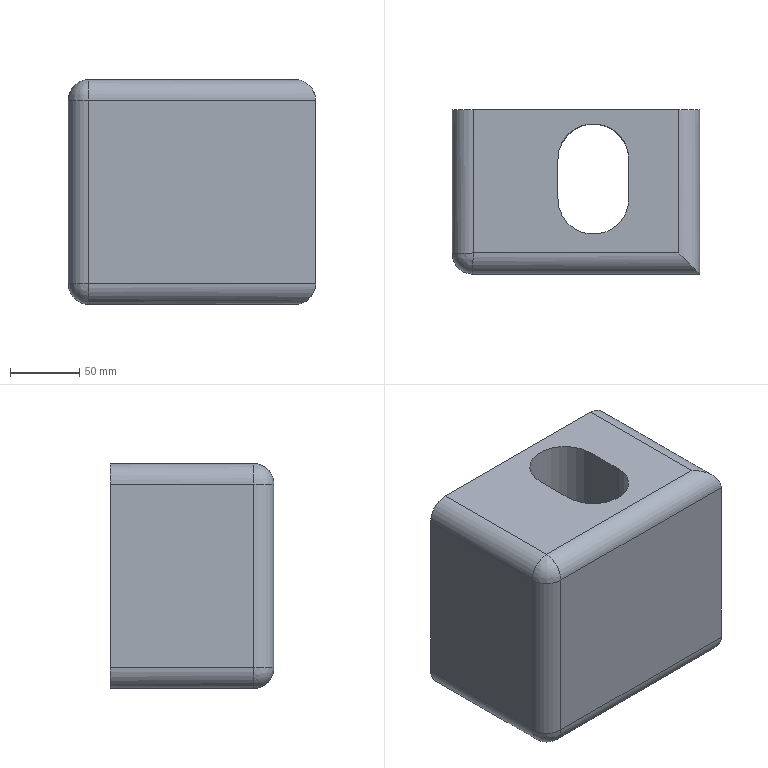Part | SolidWorks | features Extrusion 1, Fillet 1 | 1 solid | 19 faces | box 178 x 118 x 162 mm | volume 2790702 mm3 | cylinder 9 | plane 8 | spline 2 | commonest cylinder face diameters 30 x6 51 x2 29 x1
STEP:
#1=CARTESIAN_POINT('',(-163.,-103.,162.));
#2=VERTEX_POINT('',#1);
#3=CARTESIAN_POINT('',(-15.,-103.,162.));
#4=VERTEX_POINT('',#3);
#5=CARTESIAN_POINT('',(0.,-103.,162.));
#6=DIRECTION('',(1.,0.,0.));
#7=VECTOR('',#6,1000.);
#8=LINE('',#5,#7);
#9=EDGE_CURVE('',#2,#4,#8,.T.);
#10=ORIENTED_EDGE('',*,*,#9,.T.);
#11=CARTESIAN_POINT('',(-15.,0.,162.));
#12=VERTEX_POINT('',#11);
#13=CARTESIAN_POINT('',(-15.,0.,162.));
#14=DIRECTION('',(0.,1.,0.));
#15=VECTOR('',#14,1000.);
#16=LINE('',#13,#15);
#17=EDGE_CURVE('',#4,#12,#16,.T.);
#18=ORIENTED_EDGE('',*,*,#17,.T.);
#19=CARTESIAN_POINT('',(-163.,0.,162.));
#20=VERTEX_POINT('',#19);
#21=CARTESIAN_POINT('',(0.,0.,162.));
#22=DIRECTION('',(-1.,0.,0.));
#23=VECTOR('',#22,1000.);
#24=LINE('',#21,#23);
#25=EDGE_CURVE('',#12,#20,#24,.T.);
#26=ORIENTED_EDGE('',*,*,#25,.T.);
#27=CARTESIAN_POINT('',(-163.,-103.5,162.));
#28=DIRECTION('',(0.,-1.,0.));
#29=VECTOR('',#28,1000.);
#30=LINE('',#27,#29);
#31=EDGE_CURVE('',#20,#2,#30,.T.);
#32=ORIENTED_EDGE('',*,*,#31,.T.);
#33=EDGE_LOOP('',(#10,#18,#26,#32));
#34=FACE_OUTER_BOUND('',#33,.T.);
#35=CARTESIAN_POINT('',(-51.,-64.,162.));
#36=VERTEX_POINT('',#35);
#37=CARTESIAN_POINT('',(-51.,-35.5,162.));
#38=VERTEX_POINT('',#37);
#39=CARTESIAN_POINT('',(-51.,-35.5,162.));
#40=DIRECTION('',(0.,1.,0.));
#41=VECTOR('',#40,1000.);
#42=LINE('',#39,#41);
#43=EDGE_CURVE('',#36,#38,#42,.T.);
#44=ORIENTED_EDGE('',*,*,#43,.F.);
#45=CARTESIAN_POINT('',(-102.,-64.,162.));
#46=VERTEX_POINT('',#45);
#47=CARTESIAN_POINT('',(-76.5,-64.,162.));
#48=DIRECTION('',(0.,0.,1.));
#49=DIRECTION('',(1.,0.,0.));
#50=AXIS2_PLACEMENT_3D('',#47,#48,#49);
#51=CIRCLE('',#50,25.5);
#52=EDGE_CURVE('',#46,#36,#51,.T.);
#53=ORIENTED_EDGE('',*,*,#52,.F.);
#54=CARTESIAN_POINT('',(-102.,-35.5,162.));
#55=VERTEX_POINT('',#54);
#56=CARTESIAN_POINT('',(-102.,-64.,162.));
#57=DIRECTION('',(0.,-1.,0.));
#58=VECTOR('',#57,1000.);
#59=LINE('',#56,#58);
#60=EDGE_CURVE('',#55,#46,#59,.T.);
#61=ORIENTED_EDGE('',*,*,#60,.F.);
#62=CARTESIAN_POINT('',(-76.5,-35.5,162.));
#63=DIRECTION('',(0.,0.,1.));
#64=DIRECTION('',(1.,0.,0.));
#65=AXIS2_PLACEMENT_3D('',#62,#63,#64);
#66=CIRCLE('',#65,25.5);
#67=EDGE_CURVE('',#38,#55,#66,.T.);
#68=ORIENTED_EDGE('',*,*,#67,.F.);
#69=EDGE_LOOP('',(#44,#53,#61,#68));
#70=FACE_BOUND('',#69,.T.);
#71=CARTESIAN_POINT('',(-163.5,-103.5,162.));
#72=DIRECTION('',(0.,0.,1.));
#73=DIRECTION('',(1.,0.,0.));
#74=AXIS2_PLACEMENT_3D('',#71,#72,#73);
#75=PLANE('',#74);
#76=ADVANCED_FACE('',(#34,#70),#75,.T.);
#77=CARTESIAN_POINT('',(-15.,0.,0.));
#78=VERTEX_POINT('',#77);
#79=CARTESIAN_POINT('',(-163.,0.,0.));
#80=VERTEX_POINT('',#79);
#81=CARTESIAN_POINT('',(0.,0.,0.));
#82=DIRECTION('',(-1.,0.,0.));
#83=VECTOR('',#82,1000.);
#84=LINE('',#81,#83);
#85=EDGE_CURVE('',#78,#80,#84,.T.);
#86=ORIENTED_EDGE('',*,*,#85,.F.);
#87=CARTESIAN_POINT('',(-15.,-103.,0.));
#88=VERTEX_POINT('',#87);
#89=CARTESIAN_POINT('',(-15.,-103.5,0.));
#90=DIRECTION('',(0.,-1.,0.));
#91=VECTOR('',#90,1000.);
#92=LINE('',#89,#91);
#93=EDGE_CURVE('',#78,#88,#92,.T.);
#94=ORIENTED_EDGE('',*,*,#93,.T.);
#95=CARTESIAN_POINT('',(-163.,-103.,0.));
#96=VERTEX_POINT('',#95);
#97=CARTESIAN_POINT('',(-163.5,-103.,0.));
#98=DIRECTION('',(-1.,0.,0.));
#99=VECTOR('',#98,1000.);
#100=LINE('',#97,#99);
#101=EDGE_CURVE('',#88,#96,#100,.T.);
#102=ORIENTED_EDGE('',*,*,#101,.T.);
#103=CARTESIAN_POINT('',(-163.,-103.5,0.));
#104=DIRECTION('',(0.,1.,0.));
#105=VECTOR('',#104,1000.);
#106=LINE('',#103,#105);
#107=EDGE_CURVE('',#96,#80,#106,.T.);
#108=ORIENTED_EDGE('',*,*,#107,.T.);
#109=EDGE_LOOP('',(#86,#94,#102,#108));
#110=FACE_OUTER_BOUND('',#109,.T.);
#111=CARTESIAN_POINT('',(-102.,-64.,0.));
#112=VERTEX_POINT('',#111);
#113=CARTESIAN_POINT('',(-51.,-64.,0.));
#114=VERTEX_POINT('',#113);
#115=CARTESIAN_POINT('',(-76.5,-64.,0.));
#116=DIRECTION('',(0.,0.,1.));
#117=DIRECTION('',(1.,0.,0.));
#118=AXIS2_PLACEMENT_3D('',#115,#116,#117);
#119=CIRCLE('',#118,25.5);
#120=EDGE_CURVE('',#112,#114,#119,.T.);
#121=ORIENTED_EDGE('',*,*,#120,.T.);
#122=CARTESIAN_POINT('',(-51.,-35.5,0.));
#123=VERTEX_POINT('',#122);
#124=CARTESIAN_POINT('',(-51.,-35.5,0.));
#125=DIRECTION('',(0.,1.,0.));
#126=VECTOR('',#125,1000.);
#127=LINE('',#124,#126);
#128=EDGE_CURVE('',#114,#123,#127,.T.);
#129=ORIENTED_EDGE('',*,*,#128,.T.);
#130=CARTESIAN_POINT('',(-102.,-35.5,0.));
#131=VERTEX_POINT('',#130);
#132=CARTESIAN_POINT('',(-76.5,-35.5,0.));
#133=DIRECTION('',(0.,0.,1.));
#134=DIRECTION('',(1.,0.,0.));
#135=AXIS2_PLACEMENT_3D('',#132,#133,#134);
#136=CIRCLE('',#135,25.5);
#137=EDGE_CURVE('',#123,#131,#136,.T.);
#138=ORIENTED_EDGE('',*,*,#137,.T.);
#139=CARTESIAN_POINT('',(-102.,-64.,0.));
#140=DIRECTION('',(0.,-1.,0.));
#141=VECTOR('',#140,1000.);
#142=LINE('',#139,#141);
#143=EDGE_CURVE('',#131,#112,#142,.T.);
#144=ORIENTED_EDGE('',*,*,#143,.T.);
#145=EDGE_LOOP('',(#121,#129,#138,#144));
#146=FACE_BOUND('',#145,.T.);
#147=CARTESIAN_POINT('',(-163.5,-103.5,0.));
#148=DIRECTION('',(0.,0.,1.));
#149=DIRECTION('',(1.,0.,0.));
#150=AXIS2_PLACEMENT_3D('',#147,#148,#149);
#151=PLANE('',#150);
#152=ADVANCED_FACE('',(#110,#146),#151,.F.);
#153=CARTESIAN_POINT('',(-163.5,-118.,147.));
#154=VERTEX_POINT('',#153);
#155=CARTESIAN_POINT('',(-163.5,-118.,15.));
#156=VERTEX_POINT('',#155);
#157=CARTESIAN_POINT('',(-163.5,-118.,162.));
#158=DIRECTION('',(0.,0.,-1.));
#159=VECTOR('',#158,1000.);
#160=LINE('',#157,#159);
#161=EDGE_CURVE('',#154,#156,#160,.T.);
#162=ORIENTED_EDGE('',*,*,#161,.T.);
#163=CARTESIAN_POINT('',(0.,-118.,15.));
#164=VERTEX_POINT('',#163);
#165=CARTESIAN_POINT('',(-163.5,-118.,15.));
#166=DIRECTION('',(1.,0.,0.));
#167=VECTOR('',#166,1000.);
#168=LINE('',#165,#167);
#169=EDGE_CURVE('',#156,#164,#168,.T.);
#170=ORIENTED_EDGE('',*,*,#169,.T.);
#171=CARTESIAN_POINT('',(0.,-118.,147.));
#172=VERTEX_POINT('',#171);
#173=CARTESIAN_POINT('',(0.,-118.,162.));
#174=DIRECTION('',(0.,0.,-1.));
#175=VECTOR('',#174,1000.);
#176=LINE('',#173,#175);
#177=EDGE_CURVE('',#172,#164,#176,.T.);
#178=ORIENTED_EDGE('',*,*,#177,.F.);
#179=CARTESIAN_POINT('',(-163.5,-118.,147.));
#180=DIRECTION('',(-1.,0.,0.));
#181=VECTOR('',#180,1000.);
#182=LINE('',#179,#181);
#183=EDGE_CURVE('',#172,#154,#182,.T.);
#184=ORIENTED_EDGE('',*,*,#183,.T.);
#185=EDGE_LOOP('',(#162,#170,#178,#184));
#186=FACE_OUTER_BOUND('',#185,.T.);
#187=CARTESIAN_POINT('',(-163.5,-118.,162.));
#188=DIRECTION('',(0.,1.,0.));
#189=DIRECTION('',(0.,0.,1.));
#190=AXIS2_PLACEMENT_3D('',#187,#188,#189);
#191=PLANE('',#190);
#192=ADVANCED_FACE('',(#186),#191,.F.);
#193=CARTESIAN_POINT('',(0.,0.,147.));
#194=VERTEX_POINT('',#193);
#195=CARTESIAN_POINT('',(0.,0.,15.));
#196=VERTEX_POINT('',#195);
#197=CARTESIAN_POINT('',(0.,0.,162.));
#198=DIRECTION('',(0.,0.,-1.));
#199=VECTOR('',#198,1000.);
#200=LINE('',#197,#199);
#201=EDGE_CURVE('',#194,#196,#200,.T.);
#202=ORIENTED_EDGE('',*,*,#201,.F.);
#203=CARTESIAN_POINT('',(0.,-118.,147.));
#204=DIRECTION('',(0.,-1.,0.));
#205=VECTOR('',#204,1000.);
#206=LINE('',#203,#205);
#207=EDGE_CURVE('',#194,#172,#206,.T.);
#208=ORIENTED_EDGE('',*,*,#207,.T.);
#209=ORIENTED_EDGE('',*,*,#177,.T.);
#210=CARTESIAN_POINT('',(0.,-118.,15.));
#211=DIRECTION('',(0.,1.,0.));
#212=VECTOR('',#211,1000.);
#213=LINE('',#210,#212);
#214=EDGE_CURVE('',#164,#196,#213,.T.);
#215=ORIENTED_EDGE('',*,*,#214,.T.);
#216=EDGE_LOOP('',(#202,#208,#209,#215));
#217=FACE_OUTER_BOUND('',#216,.T.);
#218=CARTESIAN_POINT('',(0.,-118.,162.));
#219=DIRECTION('',(-1.,0.,0.));
#220=DIRECTION('',(0.,0.,1.));
#221=AXIS2_PLACEMENT_3D('',#218,#219,#220);
#222=PLANE('',#221);
#223=ADVANCED_FACE('',(#217),#222,.F.);
#224=ORIENTED_EDGE('',*,*,#25,.F.);
#225=CARTESIAN_POINT('',(-15.,0.,147.));
#226=DIRECTION('',(0.,1.,0.));
#227=DIRECTION('',(0.,0.,-1.));
#228=AXIS2_PLACEMENT_3D('',#225,#226,#227);
#229=CIRCLE('',#228,15.);
#230=EDGE_CURVE('',#12,#194,#229,.T.);
#231=ORIENTED_EDGE('',*,*,#230,.T.);
#232=ORIENTED_EDGE('',*,*,#201,.T.);
#233=CARTESIAN_POINT('',(-15.,0.,15.));
#234=DIRECTION('',(0.,1.,0.));
#235=DIRECTION('',(0.,0.,-1.));
#236=AXIS2_PLACEMENT_3D('',#233,#234,#235);
#237=CIRCLE('',#236,15.);
#238=EDGE_CURVE('',#196,#78,#237,.T.);
#239=ORIENTED_EDGE('',*,*,#238,.T.);
#240=ORIENTED_EDGE('',*,*,#85,.T.);
#241=CARTESIAN_POINT('',(-178.,0.,15.));
#242=VERTEX_POINT('',#241);
#243=CARTESIAN_POINT('',(-163.,0.,15.));
#244=DIRECTION('',(0.,1.,0.));
#245=DIRECTION('',(0.,0.,-1.));
#246=AXIS2_PLACEMENT_3D('',#243,#244,#245);
#247=CIRCLE('',#246,15.);
#248=EDGE_CURVE('',#80,#242,#247,.T.);
#249=ORIENTED_EDGE('',*,*,#248,.T.);
#250=CARTESIAN_POINT('',(-178.,0.,147.));
#251=VERTEX_POINT('',#250);
#252=CARTESIAN_POINT('',(-178.,0.,162.));
#253=DIRECTION('',(0.,0.,-1.));
#254=VECTOR('',#253,1000.);
#255=LINE('',#252,#254);
#256=EDGE_CURVE('',#251,#242,#255,.T.);
#257=ORIENTED_EDGE('',*,*,#256,.F.);
#258=CARTESIAN_POINT('',(-163.,0.,147.));
#259=DIRECTION('',(0.,1.,0.));
#260=DIRECTION('',(0.,0.,-1.));
#261=AXIS2_PLACEMENT_3D('',#258,#259,#260);
#262=CIRCLE('',#261,15.);
#263=EDGE_CURVE('',#251,#20,#262,.T.);
#264=ORIENTED_EDGE('',*,*,#263,.T.);
#265=EDGE_LOOP('',(#224,#231,#232,#239,#240,#249,#257,#264));
#266=FACE_OUTER_BOUND('',#265,.T.);
#267=CARTESIAN_POINT('',(0.,0.,162.));
#268=DIRECTION('',(0.,-1.,0.));
#269=DIRECTION('',(0.,0.,-1.));
#270=AXIS2_PLACEMENT_3D('',#267,#268,#269);
#271=PLANE('',#270);
#272=ADVANCED_FACE('',(#266),#271,.F.);
#273=ORIENTED_EDGE('',*,*,#256,.T.);
#274=CARTESIAN_POINT('',(-178.,-103.5,15.));
#275=VERTEX_POINT('',#274);
#276=CARTESIAN_POINT('',(-178.,0.,15.));
#277=DIRECTION('',(0.,-1.,0.));
#278=VECTOR('',#277,1000.);
#279=LINE('',#276,#278);
#280=EDGE_CURVE('',#242,#275,#279,.T.);
#281=ORIENTED_EDGE('',*,*,#280,.T.);
#282=CARTESIAN_POINT('',(-178.,-103.5,147.));
#283=VERTEX_POINT('',#282);
#284=CARTESIAN_POINT('',(-178.,-103.5,162.));
#285=DIRECTION('',(0.,0.,-1.));
#286=VECTOR('',#285,1000.);
#287=LINE('',#284,#286);
#288=EDGE_CURVE('',#283,#275,#287,.T.);
#289=ORIENTED_EDGE('',*,*,#288,.F.);
#290=CARTESIAN_POINT('',(-178.,0.,147.));
#291=DIRECTION('',(0.,1.,0.));
#292=VECTOR('',#291,1000.);
#293=LINE('',#290,#292);
#294=EDGE_CURVE('',#283,#251,#293,.T.);
#295=ORIENTED_EDGE('',*,*,#294,.T.);
#296=EDGE_LOOP('',(#273,#281,#289,#295));
#297=FACE_OUTER_BOUND('',#296,.T.);
#298=CARTESIAN_POINT('',(-178.,0.,162.));
#299=DIRECTION('',(1.,0.,0.));
#300=DIRECTION('',(0.,0.,-1.));
#301=AXIS2_PLACEMENT_3D('',#298,#299,#300);
#302=PLANE('',#301);
#303=ADVANCED_FACE('',(#297),#302,.F.);
#304=ORIENTED_EDGE('',*,*,#288,.T.);
#305=CARTESIAN_POINT('',(-163.5,-103.5,15.));
#306=DIRECTION('',(0.,0.,1.));
#307=DIRECTION('',(1.,0.,0.));
#308=AXIS2_PLACEMENT_3D('',#305,#306,#307);
#309=CIRCLE('',#308,14.5);
#310=EDGE_CURVE('',#275,#156,#309,.T.);
#311=ORIENTED_EDGE('',*,*,#310,.T.);
#312=ORIENTED_EDGE('',*,*,#161,.F.);
#313=CARTESIAN_POINT('',(-163.5,-103.5,147.));
#314=DIRECTION('',(0.,0.,-1.));
#315=DIRECTION('',(-1.,0.,0.));
#316=AXIS2_PLACEMENT_3D('',#313,#314,#315);
#317=CIRCLE('',#316,14.5);
#318=EDGE_CURVE('',#154,#283,#317,.T.);
#319=ORIENTED_EDGE('',*,*,#318,.T.);
#320=EDGE_LOOP('',(#304,#311,#312,#319));
#321=FACE_OUTER_BOUND('',#320,.T.);
#322=CARTESIAN_POINT('',(-163.5,-103.5,162.));
#323=DIRECTION('',(0.,0.,-1.));
#324=DIRECTION('',(-1.,0.,0.));
#325=AXIS2_PLACEMENT_3D('',#322,#323,#324);
#326=CYLINDRICAL_SURFACE('',#325,14.5);
#327=ADVANCED_FACE('',(#321),#326,.T.);
#328=ORIENTED_EDGE('',*,*,#120,.F.);
#329=CARTESIAN_POINT('',(-102.,-64.,162.));
#330=DIRECTION('',(0.,0.,-1.));
#331=VECTOR('',#330,1000.);
#332=LINE('',#329,#331);
#333=EDGE_CURVE('',#46,#112,#332,.T.);
#334=ORIENTED_EDGE('',*,*,#333,.F.);
#335=ORIENTED_EDGE('',*,*,#52,.T.);
#336=CARTESIAN_POINT('',(-51.,-64.,162.));
#337=DIRECTION('',(0.,0.,-1.));
#338=VECTOR('',#337,1000.);
#339=LINE('',#336,#338);
#340=EDGE_CURVE('',#36,#114,#339,.T.);
#341=ORIENTED_EDGE('',*,*,#340,.T.);
#342=EDGE_LOOP('',(#328,#334,#335,#341));
#343=FACE_OUTER_BOUND('',#342,.T.);
#344=CARTESIAN_POINT('',(-76.5,-64.,162.));
#345=DIRECTION('',(0.,0.,-1.));
#346=DIRECTION('',(-1.,0.,0.));
#347=AXIS2_PLACEMENT_3D('',#344,#345,#346);
#348=CYLINDRICAL_SURFACE('',#347,25.5);
#349=ADVANCED_FACE('',(#343),#348,.F.);
#350=ORIENTED_EDGE('',*,*,#128,.F.);
#351=ORIENTED_EDGE('',*,*,#340,.F.);
#352=ORIENTED_EDGE('',*,*,#43,.T.);
#353=CARTESIAN_POINT('',(-51.,-35.5,162.));
#354=DIRECTION('',(0.,0.,-1.));
#355=VECTOR('',#354,1000.);
#356=LINE('',#353,#355);
#357=EDGE_CURVE('',#38,#123,#356,.T.);
#358=ORIENTED_EDGE('',*,*,#357,.T.);
#359=EDGE_LOOP('',(#350,#351,#352,#358));
#360=FACE_OUTER_BOUND('',#359,.T.);
#361=CARTESIAN_POINT('',(-51.,-35.5,162.));
#362=DIRECTION('',(-1.,0.,0.));
#363=DIRECTION('',(0.,0.,1.));
#364=AXIS2_PLACEMENT_3D('',#361,#362,#363);
#365=PLANE('',#364);
#366=ADVANCED_FACE('',(#360),#365,.T.);
#367=ORIENTED_EDGE('',*,*,#137,.F.);
#368=ORIENTED_EDGE('',*,*,#357,.F.);
#369=ORIENTED_EDGE('',*,*,#67,.T.);
#370=CARTESIAN_POINT('',(-102.,-35.5,162.));
#371=DIRECTION('',(0.,0.,-1.));
#372=VECTOR('',#371,1000.);
#373=LINE('',#370,#372);
#374=EDGE_CURVE('',#55,#131,#373,.T.);
#375=ORIENTED_EDGE('',*,*,#374,.T.);
#376=EDGE_LOOP('',(#367,#368,#369,#375));
#377=FACE_OUTER_BOUND('',#376,.T.);
#378=CARTESIAN_POINT('',(-76.5,-35.5,162.));
#379=DIRECTION('',(0.,0.,-1.));
#380=DIRECTION('',(-1.,0.,0.));
#381=AXIS2_PLACEMENT_3D('',#378,#379,#380);
#382=CYLINDRICAL_SURFACE('',#381,25.5);
#383=ADVANCED_FACE('',(#377),#382,.F.);
#384=ORIENTED_EDGE('',*,*,#143,.F.);
#385=ORIENTED_EDGE('',*,*,#374,.F.);
#386=ORIENTED_EDGE('',*,*,#60,.T.);
#387=ORIENTED_EDGE('',*,*,#333,.T.);
#388=EDGE_LOOP('',(#384,#385,#386,#387));
#389=FACE_OUTER_BOUND('',#388,.T.);
#390=CARTESIAN_POINT('',(-102.,-64.,162.));
#391=DIRECTION('',(1.,0.,0.));
#392=DIRECTION('',(0.,0.,-1.));
#393=AXIS2_PLACEMENT_3D('',#390,#391,#392);
#394=PLANE('',#393);
#395=ADVANCED_FACE('',(#389),#394,.T.);
#396=ORIENTED_EDGE('',*,*,#248,.F.);
#397=ORIENTED_EDGE('',*,*,#107,.F.);
#398=CARTESIAN_POINT('',(-178.,-103.5,15.));
#399=CARTESIAN_POINT('',(-178.,-103.5,6.213));
#400=CARTESIAN_POINT('',(-171.787,-103.293,0.));
#401=CARTESIAN_POINT('',(-163.,-103.,0.));
#402=(BOUNDED_CURVE()B_SPLINE_CURVE(3,(#398,#399,#400,#401),.UNSPECIFIED.,.F.,.F.)B_SPLINE_CURVE_WITH_KNOTS((4,4),(0.,1.571),.UNSPECIFIED.)CURVE()GEOMETRIC_REPRESENTATION_ITEM()RATIONAL_B_SPLINE_CURVE((1.,0.8047,0.8047,1.))REPRESENTATION_ITEM(''));
#403=EDGE_CURVE('',#275,#96,#402,.T.);
#404=ORIENTED_EDGE('',*,*,#403,.F.);
#405=ORIENTED_EDGE('',*,*,#280,.F.);
#406=EDGE_LOOP('',(#396,#397,#404,#405));
#407=FACE_OUTER_BOUND('',#406,.T.);
#408=CARTESIAN_POINT('',(-163.,0.,15.));
#409=DIRECTION('',(0.,-1.,0.));
#410=DIRECTION('',(0.,0.,-1.));
#411=AXIS2_PLACEMENT_3D('',#408,#409,#410);
#412=CYLINDRICAL_SURFACE('',#411,15.);
#413=ADVANCED_FACE('',(#407),#412,.T.);
#414=ORIENTED_EDGE('',*,*,#310,.F.);
#415=ORIENTED_EDGE('',*,*,#403,.T.);
#416=CARTESIAN_POINT('',(-163.5,-118.,15.));
#417=CARTESIAN_POINT('',(-163.5,-118.,6.213));
#418=CARTESIAN_POINT('',(-163.293,-111.787,0.));
#419=CARTESIAN_POINT('',(-163.,-103.,0.));
#420=(BOUNDED_CURVE()B_SPLINE_CURVE(3,(#416,#417,#418,#419),.UNSPECIFIED.,.F.,.F.)B_SPLINE_CURVE_WITH_KNOTS((4,4),(0.,1.571),.UNSPECIFIED.)CURVE()GEOMETRIC_REPRESENTATION_ITEM()RATIONAL_B_SPLINE_CURVE((1.,0.8047,0.8047,1.))REPRESENTATION_ITEM(''));
#421=EDGE_CURVE('',#156,#96,#420,.T.);
#422=ORIENTED_EDGE('',*,*,#421,.F.);
#423=EDGE_LOOP('',(#414,#415,#422));
#424=FACE_OUTER_BOUND('',#423,.T.);
#425=CARTESIAN_POINT('',(-178.,-103.5,15.));
#426=CARTESIAN_POINT('',(-178.,-118.,15.));
#427=CARTESIAN_POINT('',(-163.5,-118.,15.));
#428=CARTESIAN_POINT('',(-178.,-103.5,14.509));
#429=CARTESIAN_POINT('',(-178.,-118.,14.034));
#430=CARTESIAN_POINT('',(-163.5,-118.,14.509));
#431=CARTESIAN_POINT('',(-177.976,-103.499,14.018));
#432=CARTESIAN_POINT('',(-177.929,-117.929,13.072));
#433=CARTESIAN_POINT('',(-163.499,-117.976,14.018));
#434=CARTESIAN_POINT('',(-177.88,-103.496,13.041));
#435=CARTESIAN_POINT('',(-177.653,-117.653,11.205));
#436=CARTESIAN_POINT('',(-163.496,-117.88,13.041));
#437=CARTESIAN_POINT('',(-177.808,-103.494,12.555));
#438=CARTESIAN_POINT('',(-177.45,-117.45,10.304));
#439=CARTESIAN_POINT('',(-163.494,-117.808,12.555));
#440=CARTESIAN_POINT('',(-177.616,-103.487,11.592));
#441=CARTESIAN_POINT('',(-176.934,-116.934,8.61));
#442=CARTESIAN_POINT('',(-163.487,-117.616,11.592));
#443=CARTESIAN_POINT('',(-177.497,-103.483,11.115));
#444=CARTESIAN_POINT('',(-176.625,-116.625,7.82));
#445=CARTESIAN_POINT('',(-163.483,-117.497,11.115));
#446=CARTESIAN_POINT('',(-177.212,-103.474,10.176));
#447=CARTESIAN_POINT('',(-175.932,-115.932,6.374));
#448=CARTESIAN_POINT('',(-163.474,-117.212,10.176));
#449=CARTESIAN_POINT('',(-177.046,-103.468,9.713));
#450=CARTESIAN_POINT('',(-175.552,-115.552,5.719));
#451=CARTESIAN_POINT('',(-163.468,-117.046,9.713));
#452=CARTESIAN_POINT('',(-176.67,-103.456,8.806));
#453=CARTESIAN_POINT('',(-174.75,-114.75,4.55));
#454=CARTESIAN_POINT('',(-163.456,-116.67,8.806));
#455=CARTESIAN_POINT('',(-176.46,-103.449,8.362));
#456=CARTESIAN_POINT('',(-174.332,-114.332,4.035));
#457=CARTESIAN_POINT('',(-163.449,-116.46,8.362));
#458=CARTESIAN_POINT('',(-175.997,-103.433,7.496));
#459=CARTESIAN_POINT('',(-173.485,-113.485,3.134));
#460=CARTESIAN_POINT('',(-163.433,-115.997,7.496));
#461=CARTESIAN_POINT('',(-175.745,-103.425,7.075));
#462=CARTESIAN_POINT('',(-173.057,-113.057,2.747));
#463=CARTESIAN_POINT('',(-163.425,-115.745,7.075));
#464=CARTESIAN_POINT('',(-175.199,-103.407,6.258));
#465=CARTESIAN_POINT('',(-172.21,-112.21,2.082));
#466=CARTESIAN_POINT('',(-163.407,-115.199,6.258));
#467=CARTESIAN_POINT('',(-174.907,-103.397,5.864));
#468=CARTESIAN_POINT('',(-171.791,-111.791,1.803));
#469=CARTESIAN_POINT('',(-163.397,-114.907,5.864));
#470=CARTESIAN_POINT('',(-174.284,-103.376,5.105));
#471=CARTESIAN_POINT('',(-170.975,-110.975,1.332));
#472=CARTESIAN_POINT('',(-163.376,-114.284,5.105));
#473=CARTESIAN_POINT('',(-173.954,-103.365,4.74));
#474=CARTESIAN_POINT('',(-170.578,-110.578,1.138));
#475=CARTESIAN_POINT('',(-163.365,-113.954,4.74));
#476=CARTESIAN_POINT('',(-172.912,-103.33,3.699));
#477=CARTESIAN_POINT('',(-169.437,-109.437,0.6612));
#478=CARTESIAN_POINT('',(-163.33,-112.912,3.699));
#479=CARTESIAN_POINT('',(-172.15,-103.305,3.073));
#480=CARTESIAN_POINT('',(-168.717,-108.717,0.4621));
#481=CARTESIAN_POINT('',(-163.305,-112.15,3.073));
#482=CARTESIAN_POINT('',(-170.517,-103.251,1.983));
#483=CARTESIAN_POINT('',(-167.388,-107.388,0.1981));
#484=CARTESIAN_POINT('',(-163.251,-110.517,1.983));
#485=CARTESIAN_POINT('',(-169.647,-103.222,1.518));
#486=CARTESIAN_POINT('',(-166.77,-106.77,0.1274));
#487=CARTESIAN_POINT('',(-163.222,-109.647,1.518));
#488=CARTESIAN_POINT('',(-167.833,-103.161,0.7661));
#489=CARTESIAN_POINT('',(-165.614,-105.614,0.04044));
#490=CARTESIAN_POINT('',(-163.161,-107.833,0.7661));
#491=CARTESIAN_POINT('',(-166.889,-103.13,0.4798));
#492=CARTESIAN_POINT('',(-165.068,-105.068,0.02245));
#493=CARTESIAN_POINT('',(-163.13,-106.889,0.4798));
#494=CARTESIAN_POINT('',(-164.963,-103.065,0.09669));
#495=CARTESIAN_POINT('',(-164.018,-104.018,0.002354));
#496=CARTESIAN_POINT('',(-163.065,-104.963,0.09669));
#497=CARTESIAN_POINT('',(-163.982,-103.033,0.));
#498=CARTESIAN_POINT('',(-163.507,-103.507,-0.000000019));
#499=CARTESIAN_POINT('',(-163.033,-103.982,0.));
#500=CARTESIAN_POINT('',(-163.,-103.,0.));
#501=CARTESIAN_POINT('',(-163.,-103.,0.));
#502=CARTESIAN_POINT('',(-163.,-103.,0.));
#503=(BOUNDED_SURFACE()B_SPLINE_SURFACE(3,2,((#425,#426,#427),(#428,#429,#430),(#431,#432,#433),(#434,#435,#436),(#437,#438,#439),(#440,#441,#442),(#443,#444,#445),(#446,#447,#448),(#449,#450,#451),(#452,#453,#454),(#455,#456,#457),(#458,#459,#460),(#461,#462,#463),(#464,#465,#466),(#467,#468,#469),(#470,#471,#472),(#473,#474,#475),(#476,#477,#478),(#479,#480,#481),(#482,#483,#484),(#485,#486,#487),(#488,#489,#490),(#491,#492,#493),(#494,#495,#496),(#497,#498,#499),(#500,#501,#502)),.UNSPECIFIED.,.F.,.F.,.F.)B_SPLINE_SURFACE_WITH_KNOTS((4,2,2,2,2,2,2,2,2,2,2,2,4),(3,3),(6.283,6.381,6.48,6.578,6.676,6.774,6.872,6.97,7.069,7.265,7.461,7.658,7.854),(0.,1.),.UNSPECIFIED.)GEOMETRIC_REPRESENTATION_ITEM()RATIONAL_B_SPLINE_SURFACE(((1.,0.7071,1.),(1.,0.7071,1.),(1.,0.7082,1.),(1.,0.7127,1.),(1.,0.7161,1.),(1.,0.7248,1.),(1.,0.7301,1.),(1.,0.7425,1.),(1.,0.7495,1.),(1.,0.7648,1.),(1.,0.773,1.),(1.,0.7904,1.),(1.,0.7996,1.),(1.,0.8183,1.),(1.,0.8278,1.),(1.,0.847,1.),(1.,0.8566,1.),(1.,0.8849,1.),(1.,0.9032,1.),(1.,0.936,1.),(1.,0.9507,1.),(1.,0.9747,1.),(1.,0.9841,1.),(1.,0.9968,1.),(1.,1.,1.),(1.,1.,1.)))REPRESENTATION_ITEM('')SURFACE());
#504=ADVANCED_FACE('',(#424),#503,.T.);
#505=ORIENTED_EDGE('',*,*,#238,.F.);
#506=ORIENTED_EDGE('',*,*,#214,.F.);
#507=CARTESIAN_POINT('',(-15.,-103.,0.));
#508=CARTESIAN_POINT('',(-6.213,-111.787,0.));
#509=CARTESIAN_POINT('',(0.,-118.,6.213));
#510=CARTESIAN_POINT('',(0.,-118.,15.));
#511=(BOUNDED_CURVE()B_SPLINE_CURVE(3,(#507,#508,#509,#510),.UNSPECIFIED.,.F.,.F.)B_SPLINE_CURVE_WITH_KNOTS((4,4),(1.571,3.142),.UNSPECIFIED.)CURVE()GEOMETRIC_REPRESENTATION_ITEM()RATIONAL_B_SPLINE_CURVE((1.,0.8047,0.8047,1.))REPRESENTATION_ITEM(''));
#512=EDGE_CURVE('',#88,#164,#511,.T.);
#513=ORIENTED_EDGE('',*,*,#512,.F.);
#514=ORIENTED_EDGE('',*,*,#93,.F.);
#515=EDGE_LOOP('',(#505,#506,#513,#514));
#516=FACE_OUTER_BOUND('',#515,.T.);
#517=CARTESIAN_POINT('',(-15.,-118.,15.));
#518=DIRECTION('',(0.,1.,0.));
#519=DIRECTION('',(0.,0.,1.));
#520=AXIS2_PLACEMENT_3D('',#517,#518,#519);
#521=CYLINDRICAL_SURFACE('',#520,15.);
#522=ADVANCED_FACE('',(#516),#521,.T.);
#523=ORIENTED_EDGE('',*,*,#421,.T.);
#524=ORIENTED_EDGE('',*,*,#101,.F.);
#525=ORIENTED_EDGE('',*,*,#512,.T.);
#526=ORIENTED_EDGE('',*,*,#169,.F.);
#527=EDGE_LOOP('',(#523,#524,#525,#526));
#528=FACE_OUTER_BOUND('',#527,.T.);
#529=CARTESIAN_POINT('',(-163.5,-103.,15.));
#530=DIRECTION('',(1.,0.,0.));
#531=DIRECTION('',(0.,0.,-1.));
#532=AXIS2_PLACEMENT_3D('',#529,#530,#531);
#533=CYLINDRICAL_SURFACE('',#532,15.);
#534=ADVANCED_FACE('',(#528),#533,.T.);
#535=ORIENTED_EDGE('',*,*,#263,.F.);
#536=ORIENTED_EDGE('',*,*,#294,.F.);
#537=CARTESIAN_POINT('',(-163.,-103.,162.));
#538=CARTESIAN_POINT('',(-171.787,-103.293,162.));
#539=CARTESIAN_POINT('',(-178.,-103.5,155.787));
#540=CARTESIAN_POINT('',(-178.,-103.5,147.));
#541=(BOUNDED_CURVE()B_SPLINE_CURVE(3,(#537,#538,#539,#540),.UNSPECIFIED.,.F.,.F.)B_SPLINE_CURVE_WITH_KNOTS((4,4),(4.712,6.283),.UNSPECIFIED.)CURVE()GEOMETRIC_REPRESENTATION_ITEM()RATIONAL_B_SPLINE_CURVE((1.,0.8047,0.8047,1.))REPRESENTATION_ITEM(''));
#542=EDGE_CURVE('',#2,#283,#541,.T.);
#543=ORIENTED_EDGE('',*,*,#542,.F.);
#544=ORIENTED_EDGE('',*,*,#31,.F.);
#545=EDGE_LOOP('',(#535,#536,#543,#544));
#546=FACE_OUTER_BOUND('',#545,.T.);
#547=CARTESIAN_POINT('',(-163.,-103.5,147.));
#548=DIRECTION('',(0.,1.,0.));
#549=DIRECTION('',(0.,0.,1.));
#550=AXIS2_PLACEMENT_3D('',#547,#548,#549);
#551=CYLINDRICAL_SURFACE('',#550,15.);
#552=ADVANCED_FACE('',(#546),#551,.T.);
#553=ORIENTED_EDGE('',*,*,#542,.T.);
#554=ORIENTED_EDGE('',*,*,#318,.F.);
#555=CARTESIAN_POINT('',(-163.,-103.,162.));
#556=CARTESIAN_POINT('',(-163.293,-111.787,162.));
#557=CARTESIAN_POINT('',(-163.5,-118.,155.787));
#558=CARTESIAN_POINT('',(-163.5,-118.,147.));
#559=(BOUNDED_CURVE()B_SPLINE_CURVE(3,(#555,#556,#557,#558),.UNSPECIFIED.,.F.,.F.)B_SPLINE_CURVE_WITH_KNOTS((4,4),(4.712,6.283),.UNSPECIFIED.)CURVE()GEOMETRIC_REPRESENTATION_ITEM()RATIONAL_B_SPLINE_CURVE((1.,0.8047,0.8047,1.))REPRESENTATION_ITEM(''));
#560=EDGE_CURVE('',#2,#154,#559,.T.);
#561=ORIENTED_EDGE('',*,*,#560,.F.);
#562=EDGE_LOOP('',(#553,#554,#561));
#563=FACE_OUTER_BOUND('',#562,.T.);
#564=CARTESIAN_POINT('',(-163.5,-118.,147.));
#565=CARTESIAN_POINT('',(-178.,-118.,147.));
#566=CARTESIAN_POINT('',(-178.,-103.5,147.));
#567=CARTESIAN_POINT('',(-163.5,-118.,147.491));
#568=CARTESIAN_POINT('',(-178.,-118.,147.966));
#569=CARTESIAN_POINT('',(-178.,-103.5,147.491));
#570=CARTESIAN_POINT('',(-163.499,-117.976,147.982));
#571=CARTESIAN_POINT('',(-177.929,-117.929,148.928));
#572=CARTESIAN_POINT('',(-177.976,-103.499,147.982));
#573=CARTESIAN_POINT('',(-163.496,-117.88,148.959));
#574=CARTESIAN_POINT('',(-177.653,-117.653,150.795));
#575=CARTESIAN_POINT('',(-177.88,-103.496,148.959));
#576=CARTESIAN_POINT('',(-163.494,-117.808,149.445));
#577=CARTESIAN_POINT('',(-177.45,-117.45,151.696));
#578=CARTESIAN_POINT('',(-177.808,-103.494,149.445));
#579=CARTESIAN_POINT('',(-163.487,-117.616,150.408));
#580=CARTESIAN_POINT('',(-176.934,-116.934,153.39));
#581=CARTESIAN_POINT('',(-177.616,-103.487,150.408));
#582=CARTESIAN_POINT('',(-163.483,-117.497,150.885));
#583=CARTESIAN_POINT('',(-176.625,-116.625,154.18));
#584=CARTESIAN_POINT('',(-177.497,-103.483,150.885));
#585=CARTESIAN_POINT('',(-163.474,-117.212,151.824));
#586=CARTESIAN_POINT('',(-175.932,-115.932,155.626));
#587=CARTESIAN_POINT('',(-177.212,-103.474,151.824));
#588=CARTESIAN_POINT('',(-163.468,-117.046,152.287));
#589=CARTESIAN_POINT('',(-175.552,-115.552,156.281));
#590=CARTESIAN_POINT('',(-177.046,-103.468,152.287));
#591=CARTESIAN_POINT('',(-163.456,-116.67,153.194));
#592=CARTESIAN_POINT('',(-174.75,-114.75,157.45));
#593=CARTESIAN_POINT('',(-176.67,-103.456,153.194));
#594=CARTESIAN_POINT('',(-163.449,-116.46,153.638));
#595=CARTESIAN_POINT('',(-174.332,-114.332,157.965));
#596=CARTESIAN_POINT('',(-176.46,-103.449,153.638));
#597=CARTESIAN_POINT('',(-163.433,-115.997,154.504));
#598=CARTESIAN_POINT('',(-173.485,-113.485,158.866));
#599=CARTESIAN_POINT('',(-175.997,-103.433,154.504));
#600=CARTESIAN_POINT('',(-163.425,-115.745,154.925));
#601=CARTESIAN_POINT('',(-173.057,-113.057,159.253));
#602=CARTESIAN_POINT('',(-175.745,-103.425,154.925));
#603=CARTESIAN_POINT('',(-163.407,-115.199,155.742));
#604=CARTESIAN_POINT('',(-172.21,-112.21,159.918));
#605=CARTESIAN_POINT('',(-175.199,-103.407,155.742));
#606=CARTESIAN_POINT('',(-163.397,-114.907,156.136));
#607=CARTESIAN_POINT('',(-171.791,-111.791,160.197));
#608=CARTESIAN_POINT('',(-174.907,-103.397,156.136));
#609=CARTESIAN_POINT('',(-163.376,-114.284,156.895));
#610=CARTESIAN_POINT('',(-170.975,-110.975,160.668));
#611=CARTESIAN_POINT('',(-174.284,-103.376,156.895));
#612=CARTESIAN_POINT('',(-163.365,-113.954,157.26));
#613=CARTESIAN_POINT('',(-170.578,-110.578,160.862));
#614=CARTESIAN_POINT('',(-173.954,-103.365,157.26));
#615=CARTESIAN_POINT('',(-163.33,-112.912,158.301));
#616=CARTESIAN_POINT('',(-169.437,-109.437,161.339));
#617=CARTESIAN_POINT('',(-172.912,-103.33,158.301));
#618=CARTESIAN_POINT('',(-163.305,-112.15,158.927));
#619=CARTESIAN_POINT('',(-168.717,-108.717,161.538));
#620=CARTESIAN_POINT('',(-172.15,-103.305,158.927));
#621=CARTESIAN_POINT('',(-163.251,-110.517,160.017));
#622=CARTESIAN_POINT('',(-167.388,-107.388,161.802));
#623=CARTESIAN_POINT('',(-170.517,-103.251,160.017));
#624=CARTESIAN_POINT('',(-163.222,-109.647,160.482));
#625=CARTESIAN_POINT('',(-166.77,-106.77,161.873));
#626=CARTESIAN_POINT('',(-169.647,-103.222,160.482));
#627=CARTESIAN_POINT('',(-163.161,-107.833,161.234));
#628=CARTESIAN_POINT('',(-165.614,-105.614,161.96));
#629=CARTESIAN_POINT('',(-167.833,-103.161,161.234));
#630=CARTESIAN_POINT('',(-163.13,-106.889,161.52));
#631=CARTESIAN_POINT('',(-165.068,-105.068,161.978));
#632=CARTESIAN_POINT('',(-166.889,-103.13,161.52));
#633=CARTESIAN_POINT('',(-163.065,-104.963,161.903));
#634=CARTESIAN_POINT('',(-164.018,-104.018,161.998));
#635=CARTESIAN_POINT('',(-164.963,-103.065,161.903));
#636=CARTESIAN_POINT('',(-163.033,-103.982,162.));
#637=CARTESIAN_POINT('',(-163.507,-103.507,162.));
#638=CARTESIAN_POINT('',(-163.982,-103.033,162.));
#639=CARTESIAN_POINT('',(-163.,-103.,162.));
#640=CARTESIAN_POINT('',(-163.,-103.,162.));
#641=CARTESIAN_POINT('',(-163.,-103.,162.));
#642=(BOUNDED_SURFACE()B_SPLINE_SURFACE(3,2,((#564,#565,#566),(#567,#568,#569),(#570,#571,#572),(#573,#574,#575),(#576,#577,#578),(#579,#580,#581),(#582,#583,#584),(#585,#586,#587),(#588,#589,#590),(#591,#592,#593),(#594,#595,#596),(#597,#598,#599),(#600,#601,#602),(#603,#604,#605),(#606,#607,#608),(#609,#610,#611),(#612,#613,#614),(#615,#616,#617),(#618,#619,#620),(#621,#622,#623),(#624,#625,#626),(#627,#628,#629),(#630,#631,#632),(#633,#634,#635),(#636,#637,#638),(#639,#640,#641)),.UNSPECIFIED.,.F.,.F.,.F.)B_SPLINE_SURFACE_WITH_KNOTS((4,2,2,2,2,2,2,2,2,2,2,2,4),(3,3),(6.283,6.381,6.48,6.578,6.676,6.774,6.872,6.97,7.069,7.265,7.461,7.658,7.854),(0.,1.),.UNSPECIFIED.)GEOMETRIC_REPRESENTATION_ITEM()RATIONAL_B_SPLINE_SURFACE(((1.,0.7071,1.),(1.,0.7071,1.),(1.,0.7082,1.),(1.,0.7127,1.),(1.,0.7161,1.),(1.,0.7248,1.),(1.,0.7301,1.),(1.,0.7425,1.),(1.,0.7495,1.),(1.,0.7648,1.),(1.,0.773,1.),(1.,0.7904,1.),(1.,0.7996,1.),(1.,0.8183,1.),(1.,0.8278,1.),(1.,0.847,1.),(1.,0.8566,1.),(1.,0.8849,1.),(1.,0.9032,1.),(1.,0.936,1.),(1.,0.9507,1.),(1.,0.9747,1.),(1.,0.9841,1.),(1.,0.9968,1.),(1.,1.,1.),(1.,1.,1.)))REPRESENTATION_ITEM('')SURFACE());
#643=ADVANCED_FACE('',(#563),#642,.T.);
#644=ORIENTED_EDGE('',*,*,#230,.F.);
#645=ORIENTED_EDGE('',*,*,#17,.F.);
#646=CARTESIAN_POINT('',(0.,-118.,147.));
#647=CARTESIAN_POINT('',(0.,-118.,155.787));
#648=CARTESIAN_POINT('',(-6.213,-111.787,162.));
#649=CARTESIAN_POINT('',(-15.,-103.,162.));
#650=(BOUNDED_CURVE()B_SPLINE_CURVE(3,(#646,#647,#648,#649),.UNSPECIFIED.,.F.,.F.)B_SPLINE_CURVE_WITH_KNOTS((4,4),(0.,1.571),.UNSPECIFIED.)CURVE()GEOMETRIC_REPRESENTATION_ITEM()RATIONAL_B_SPLINE_CURVE((1.,0.8047,0.8047,1.))REPRESENTATION_ITEM(''));
#651=EDGE_CURVE('',#172,#4,#650,.T.);
#652=ORIENTED_EDGE('',*,*,#651,.F.);
#653=ORIENTED_EDGE('',*,*,#207,.F.);
#654=EDGE_LOOP('',(#644,#645,#652,#653));
#655=FACE_OUTER_BOUND('',#654,.T.);
#656=CARTESIAN_POINT('',(-15.,-103.5,147.));
#657=DIRECTION('',(0.,-1.,0.));
#658=DIRECTION('',(0.,0.,-1.));
#659=AXIS2_PLACEMENT_3D('',#656,#657,#658);
#660=CYLINDRICAL_SURFACE('',#659,15.);
#661=ADVANCED_FACE('',(#655),#660,.T.);
#662=ORIENTED_EDGE('',*,*,#560,.T.);
#663=ORIENTED_EDGE('',*,*,#183,.F.);
#664=ORIENTED_EDGE('',*,*,#651,.T.);
#665=ORIENTED_EDGE('',*,*,#9,.F.);
#666=EDGE_LOOP('',(#662,#663,#664,#665));
#667=FACE_OUTER_BOUND('',#666,.T.);
#668=CARTESIAN_POINT('',(-163.5,-103.,147.));
#669=DIRECTION('',(-1.,0.,0.));
#670=DIRECTION('',(0.,0.,1.));
#671=AXIS2_PLACEMENT_3D('',#668,#669,#670);
#672=CYLINDRICAL_SURFACE('',#671,15.);
#673=ADVANCED_FACE('',(#667),#672,.T.);
#674=CLOSED_SHELL('',(#76,#152,#192,#223,#272,#303,#327,#349,#366,#383,#395,#413,#504,#522,#534,#552,#643,#661,#673));
#675=MANIFOLD_SOLID_BREP('',#674);
#676=CARTESIAN_POINT('',(0.,0.,0.));
#677=DIRECTION('',(0.,0.,1.));
#678=DIRECTION('',(1.,0.,0.));
#679=AXIS2_PLACEMENT_3D('',#676,#677,#678);
#680=(LENGTH_UNIT()NAMED_UNIT(*)SI_UNIT(.MILLI.,.METRE.));
#681=UNCERTAINTY_MEASURE_WITH_UNIT(LENGTH_MEASURE(0.00001),#680,'','');
#682=(NAMED_UNIT(*)PLANE_ANGLE_UNIT()SI_UNIT($,.RADIAN.));
#683=(NAMED_UNIT(*)SI_UNIT($,.STERADIAN.)SOLID_ANGLE_UNIT());
#684=(GEOMETRIC_REPRESENTATION_CONTEXT(3)GLOBAL_UNCERTAINTY_ASSIGNED_CONTEXT((#681))GLOBAL_UNIT_ASSIGNED_CONTEXT((#680,#682,#683))REPRESENTATION_CONTEXT('',''));
#685=ADVANCED_BREP_SHAPE_REPRESENTATION('',(#675,#679),#684);